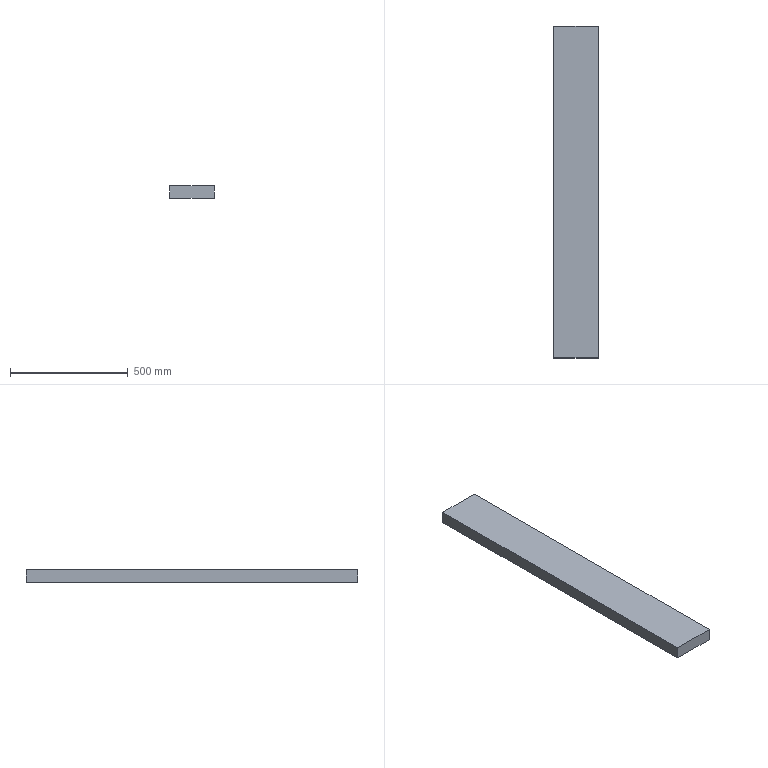Part | SolidWorks | features BaseBody 1 | 1 solid | 6 faces | box 190 x 1410 x 53 mm | volume 14198700 mm3 | plane 6
STEP:
#1=CARTESIAN_POINT('',(-95.,705.,-26.5));
#2=VERTEX_POINT('',#1);
#3=CARTESIAN_POINT('',(-95.,-705.,-26.5));
#4=VERTEX_POINT('',#3);
#5=CARTESIAN_POINT('',(-95.,-705.,-26.5));
#6=DIRECTION('',(0.,-1.,0.));
#7=VECTOR('',#6,1000.);
#8=LINE('',#5,#7);
#9=EDGE_CURVE('',#2,#4,#8,.T.);
#10=ORIENTED_EDGE('',*,*,#9,.T.);
#11=CARTESIAN_POINT('',(-95.,-705.,26.5));
#12=VERTEX_POINT('',#11);
#13=CARTESIAN_POINT('',(-95.,-705.,26.5));
#14=DIRECTION('',(0.,0.,-1.));
#15=VECTOR('',#14,1000.);
#16=LINE('',#13,#15);
#17=EDGE_CURVE('',#12,#4,#16,.T.);
#18=ORIENTED_EDGE('',*,*,#17,.F.);
#19=CARTESIAN_POINT('',(-95.,705.,26.5));
#20=VERTEX_POINT('',#19);
#21=CARTESIAN_POINT('',(-95.,-705.,26.5));
#22=DIRECTION('',(0.,-1.,0.));
#23=VECTOR('',#22,1000.);
#24=LINE('',#21,#23);
#25=EDGE_CURVE('',#20,#12,#24,.T.);
#26=ORIENTED_EDGE('',*,*,#25,.F.);
#27=CARTESIAN_POINT('',(-95.,705.,26.5));
#28=DIRECTION('',(0.,0.,-1.));
#29=VECTOR('',#28,1000.);
#30=LINE('',#27,#29);
#31=EDGE_CURVE('',#20,#2,#30,.T.);
#32=ORIENTED_EDGE('',*,*,#31,.T.);
#33=EDGE_LOOP('',(#10,#18,#26,#32));
#34=FACE_OUTER_BOUND('',#33,.T.);
#35=CARTESIAN_POINT('',(-95.,-705.,26.5));
#36=DIRECTION('',(1.,0.,0.));
#37=DIRECTION('',(0.,0.,-1.));
#38=AXIS2_PLACEMENT_3D('',#35,#36,#37);
#39=PLANE('',#38);
#40=ADVANCED_FACE('',(#34),#39,.F.);
#41=CARTESIAN_POINT('',(95.,-705.,-26.5));
#42=VERTEX_POINT('',#41);
#43=CARTESIAN_POINT('',(95.,-705.,-26.5));
#44=DIRECTION('',(1.,0.,0.));
#45=VECTOR('',#44,1000.);
#46=LINE('',#43,#45);
#47=EDGE_CURVE('',#4,#42,#46,.T.);
#48=ORIENTED_EDGE('',*,*,#47,.T.);
#49=CARTESIAN_POINT('',(95.,-705.,26.5));
#50=VERTEX_POINT('',#49);
#51=CARTESIAN_POINT('',(95.,-705.,26.5));
#52=DIRECTION('',(0.,0.,-1.));
#53=VECTOR('',#52,1000.);
#54=LINE('',#51,#53);
#55=EDGE_CURVE('',#50,#42,#54,.T.);
#56=ORIENTED_EDGE('',*,*,#55,.F.);
#57=CARTESIAN_POINT('',(95.,-705.,26.5));
#58=DIRECTION('',(1.,0.,0.));
#59=VECTOR('',#58,1000.);
#60=LINE('',#57,#59);
#61=EDGE_CURVE('',#12,#50,#60,.T.);
#62=ORIENTED_EDGE('',*,*,#61,.F.);
#63=ORIENTED_EDGE('',*,*,#17,.T.);
#64=EDGE_LOOP('',(#48,#56,#62,#63));
#65=FACE_OUTER_BOUND('',#64,.T.);
#66=CARTESIAN_POINT('',(95.,-705.,26.5));
#67=DIRECTION('',(0.,1.,0.));
#68=DIRECTION('',(0.,0.,1.));
#69=AXIS2_PLACEMENT_3D('',#66,#67,#68);
#70=PLANE('',#69);
#71=ADVANCED_FACE('',(#65),#70,.F.);
#72=CARTESIAN_POINT('',(95.,705.,-26.5));
#73=VERTEX_POINT('',#72);
#74=CARTESIAN_POINT('',(95.,-705.,-26.5));
#75=DIRECTION('',(0.,1.,0.));
#76=VECTOR('',#75,1000.);
#77=LINE('',#74,#76);
#78=EDGE_CURVE('',#42,#73,#77,.T.);
#79=ORIENTED_EDGE('',*,*,#78,.T.);
#80=CARTESIAN_POINT('',(95.,705.,26.5));
#81=VERTEX_POINT('',#80);
#82=CARTESIAN_POINT('',(95.,705.,26.5));
#83=DIRECTION('',(0.,0.,-1.));
#84=VECTOR('',#83,1000.);
#85=LINE('',#82,#84);
#86=EDGE_CURVE('',#81,#73,#85,.T.);
#87=ORIENTED_EDGE('',*,*,#86,.F.);
#88=CARTESIAN_POINT('',(95.,-705.,26.5));
#89=DIRECTION('',(0.,1.,0.));
#90=VECTOR('',#89,1000.);
#91=LINE('',#88,#90);
#92=EDGE_CURVE('',#50,#81,#91,.T.);
#93=ORIENTED_EDGE('',*,*,#92,.F.);
#94=ORIENTED_EDGE('',*,*,#55,.T.);
#95=EDGE_LOOP('',(#79,#87,#93,#94));
#96=FACE_OUTER_BOUND('',#95,.T.);
#97=CARTESIAN_POINT('',(95.,-705.,26.5));
#98=DIRECTION('',(-1.,0.,0.));
#99=DIRECTION('',(0.,0.,1.));
#100=AXIS2_PLACEMENT_3D('',#97,#98,#99);
#101=PLANE('',#100);
#102=ADVANCED_FACE('',(#96),#101,.F.);
#103=CARTESIAN_POINT('',(95.,705.,-26.5));
#104=DIRECTION('',(-1.,0.,0.));
#105=VECTOR('',#104,1000.);
#106=LINE('',#103,#105);
#107=EDGE_CURVE('',#73,#2,#106,.T.);
#108=ORIENTED_EDGE('',*,*,#107,.T.);
#109=ORIENTED_EDGE('',*,*,#31,.F.);
#110=CARTESIAN_POINT('',(95.,705.,26.5));
#111=DIRECTION('',(-1.,0.,0.));
#112=VECTOR('',#111,1000.);
#113=LINE('',#110,#112);
#114=EDGE_CURVE('',#81,#20,#113,.T.);
#115=ORIENTED_EDGE('',*,*,#114,.F.);
#116=ORIENTED_EDGE('',*,*,#86,.T.);
#117=EDGE_LOOP('',(#108,#109,#115,#116));
#118=FACE_OUTER_BOUND('',#117,.T.);
#119=CARTESIAN_POINT('',(95.,705.,26.5));
#120=DIRECTION('',(0.,-1.,0.));
#121=DIRECTION('',(0.,0.,-1.));
#122=AXIS2_PLACEMENT_3D('',#119,#120,#121);
#123=PLANE('',#122);
#124=ADVANCED_FACE('',(#118),#123,.F.);
#125=ORIENTED_EDGE('',*,*,#25,.T.);
#126=ORIENTED_EDGE('',*,*,#61,.T.);
#127=ORIENTED_EDGE('',*,*,#92,.T.);
#128=ORIENTED_EDGE('',*,*,#114,.T.);
#129=EDGE_LOOP('',(#125,#126,#127,#128));
#130=FACE_OUTER_BOUND('',#129,.T.);
#131=CARTESIAN_POINT('',(0.,0.,26.5));
#132=DIRECTION('',(0.,0.,1.));
#133=DIRECTION('',(1.,0.,0.));
#134=AXIS2_PLACEMENT_3D('',#131,#132,#133);
#135=PLANE('',#134);
#136=ADVANCED_FACE('',(#130),#135,.T.);
#137=ORIENTED_EDGE('',*,*,#9,.F.);
#138=ORIENTED_EDGE('',*,*,#107,.F.);
#139=ORIENTED_EDGE('',*,*,#78,.F.);
#140=ORIENTED_EDGE('',*,*,#47,.F.);
#141=EDGE_LOOP('',(#137,#138,#139,#140));
#142=FACE_OUTER_BOUND('',#141,.T.);
#143=CARTESIAN_POINT('',(0.,0.,-26.5));
#144=DIRECTION('',(0.,0.,1.));
#145=DIRECTION('',(1.,0.,0.));
#146=AXIS2_PLACEMENT_3D('',#143,#144,#145);
#147=PLANE('',#146);
#148=ADVANCED_FACE('',(#142),#147,.F.);
#149=CLOSED_SHELL('',(#40,#71,#102,#124,#136,#148));
#150=MANIFOLD_SOLID_BREP('',#149);
#151=CARTESIAN_POINT('',(0.,0.,0.));
#152=DIRECTION('',(0.,0.,1.));
#153=DIRECTION('',(1.,0.,0.));
#154=AXIS2_PLACEMENT_3D('',#151,#152,#153);
#155=(LENGTH_UNIT()NAMED_UNIT(*)SI_UNIT(.MILLI.,.METRE.));
#156=UNCERTAINTY_MEASURE_WITH_UNIT(LENGTH_MEASURE(0.00001),#155,'','');
#157=(NAMED_UNIT(*)PLANE_ANGLE_UNIT()SI_UNIT($,.RADIAN.));
#158=(NAMED_UNIT(*)SI_UNIT($,.STERADIAN.)SOLID_ANGLE_UNIT());
#159=(GEOMETRIC_REPRESENTATION_CONTEXT(3)GLOBAL_UNCERTAINTY_ASSIGNED_CONTEXT((#156))GLOBAL_UNIT_ASSIGNED_CONTEXT((#155,#157,#158))REPRESENTATION_CONTEXT('',''));
#160=ADVANCED_BREP_SHAPE_REPRESENTATION('',(#150,#154),#159);